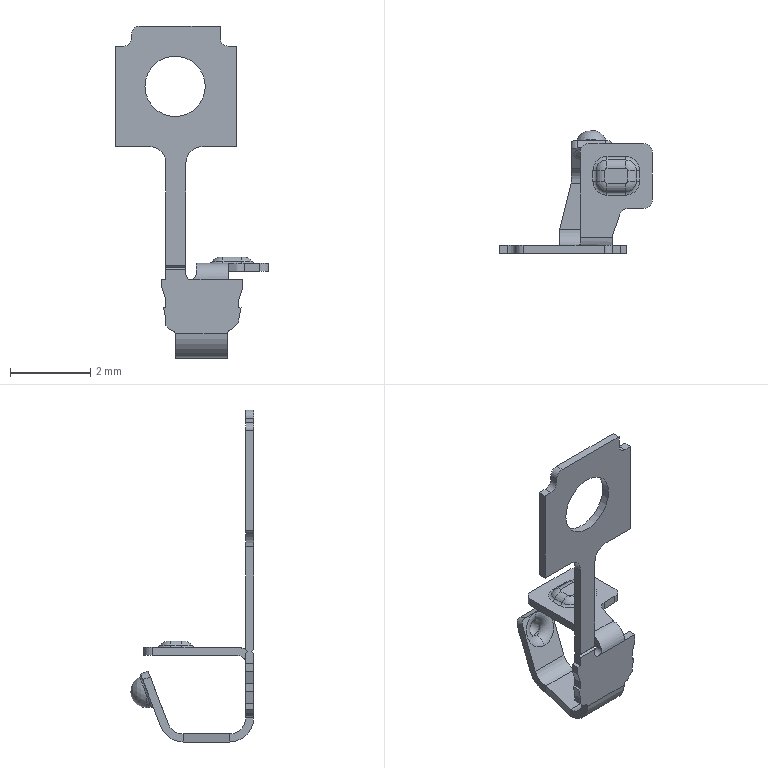Part | NX | 1 solid | 118 faces | box 3.8 x 3.065 x 8.25 mm | volume 3.955 mm3 | plane 54 | cylinder 40 | torus 20 | sphere 4 | commonest cylinder face diameters 0.2 x8 0.8 x5 0.12 x4 0.4 x4 0.44 x4 0.52 x4